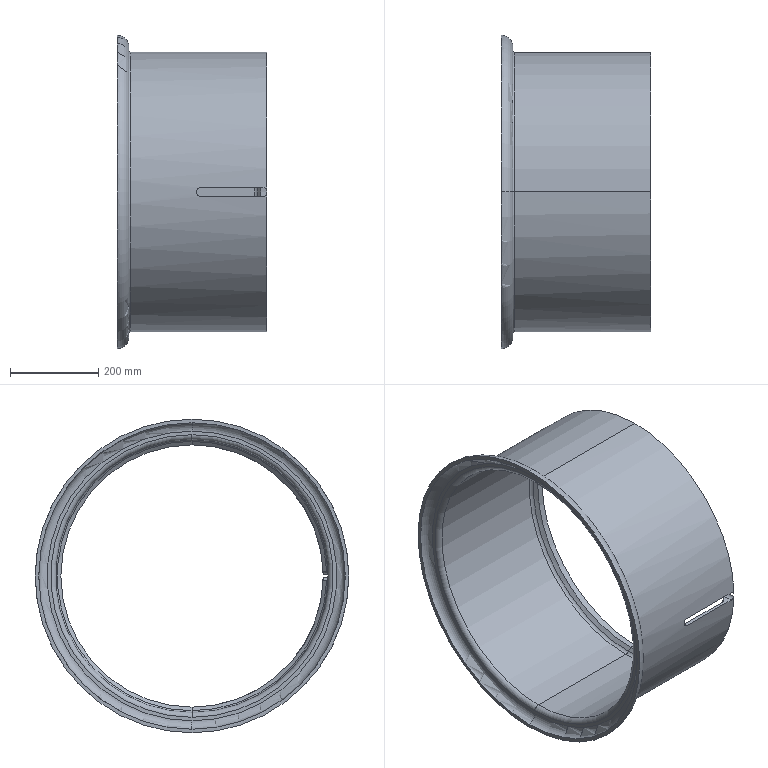Part | SolidWorks | features Fillet 2, ICE 1, Revolution 1 | 1 solid | 30 faces | box 340 x 711 x 711 mm | volume 6226699 mm3 | torus 11 | cylinder 10 | plane 6 | cone 3 | commonest cylinder face diameters 20 x3 595 x3 619 x2 635 x2
STEP:
#1=CARTESIAN_POINT('',(27.,0.,-320.5));
#2=VERTEX_POINT('',#1);
#3=CARTESIAN_POINT('',(27.,0.,320.5));
#4=VERTEX_POINT('',#3);
#5=CARTESIAN_POINT('',(27.,0.,0.));
#6=DIRECTION('',(-1.,0.,0.));
#7=DIRECTION('',(0.,0.,1.));
#8=AXIS2_PLACEMENT_3D('',#5,#6,#7);
#9=CIRCLE('',#8,320.5);
#10=EDGE_CURVE('',#2,#4,#9,.T.);
#11=ORIENTED_EDGE('',*,*,#10,.F.);
#12=CARTESIAN_POINT('',(30.,0.,-317.5));
#13=VERTEX_POINT('',#12);
#14=CARTESIAN_POINT('',(30.,0.,-320.5));
#15=DIRECTION('',(0.,1.,0.));
#16=DIRECTION('',(0.,0.,1.));
#17=AXIS2_PLACEMENT_3D('',#14,#15,#16);
#18=CIRCLE('',#17,3.);
#19=EDGE_CURVE('',#2,#13,#18,.T.);
#20=ORIENTED_EDGE('',*,*,#19,.T.);
#21=CARTESIAN_POINT('',(30.,0.,317.5));
#22=VERTEX_POINT('',#21);
#23=CARTESIAN_POINT('',(30.,0.,0.));
#24=DIRECTION('',(1.,0.,0.));
#25=DIRECTION('',(0.,0.,1.));
#26=AXIS2_PLACEMENT_3D('',#23,#24,#25);
#27=CIRCLE('',#26,317.5);
#28=EDGE_CURVE('',#22,#13,#27,.T.);
#29=ORIENTED_EDGE('',*,*,#28,.F.);
#30=CARTESIAN_POINT('',(30.,0.,320.5));
#31=DIRECTION('',(0.,-1.,0.));
#32=DIRECTION('',(0.,0.,-1.));
#33=AXIS2_PLACEMENT_3D('',#30,#31,#32);
#34=CIRCLE('',#33,3.);
#35=EDGE_CURVE('',#4,#22,#34,.T.);
#36=ORIENTED_EDGE('',*,*,#35,.F.);
#37=EDGE_LOOP('',(#11,#20,#29,#36));
#38=FACE_OUTER_BOUND('',#37,.T.);
#39=CARTESIAN_POINT('',(30.,0.,0.));
#40=DIRECTION('',(-1.,0.,0.));
#41=DIRECTION('',(0.,0.,1.));
#42=AXIS2_PLACEMENT_3D('',#39,#40,#41);
#43=TOROIDAL_SURFACE('',#42,320.5,3.);
#44=ADVANCED_FACE('',(#38),#43,.F.);
#45=CARTESIAN_POINT('',(319.298,0.,-305.542));
#46=VERTEX_POINT('',#45);
#47=CARTESIAN_POINT('',(319.298,-305.378,-10.));
#48=VERTEX_POINT('',#47);
#49=CARTESIAN_POINT('',(319.298,0.,0.));
#50=DIRECTION('',(-1.,0.,0.));
#51=DIRECTION('',(0.,0.,1.));
#52=AXIS2_PLACEMENT_3D('',#49,#50,#51);
#53=CIRCLE('',#52,305.542);
#54=EDGE_CURVE('',#46,#48,#53,.T.);
#55=ORIENTED_EDGE('',*,*,#54,.F.);
#56=CARTESIAN_POINT('',(310.848,0.,-309.5));
#57=VERTEX_POINT('',#56);
#58=CARTESIAN_POINT('',(310.848,0.,-298.5));
#59=DIRECTION('',(0.,1.,0.));
#60=DIRECTION('',(0.,0.,1.));
#61=AXIS2_PLACEMENT_3D('',#58,#59,#60);
#62=CIRCLE('',#61,11.);
#63=EDGE_CURVE('',#46,#57,#62,.T.);
#64=ORIENTED_EDGE('',*,*,#63,.T.);
#65=CARTESIAN_POINT('',(310.848,-309.338,-10.));
#66=VERTEX_POINT('',#65);
#67=CARTESIAN_POINT('',(310.848,0.,0.));
#68=DIRECTION('',(1.,0.,0.));
#69=DIRECTION('',(0.,0.,1.));
#70=AXIS2_PLACEMENT_3D('',#67,#68,#69);
#71=CIRCLE('',#70,309.5);
#72=EDGE_CURVE('',#66,#57,#71,.T.);
#73=ORIENTED_EDGE('',*,*,#72,.F.);
#74=CARTESIAN_POINT('',(310.848,-309.338,-10.));
#75=CARTESIAN_POINT('',(311.247,-309.338,-10.));
#76=CARTESIAN_POINT('',(311.646,-309.317,-10.));
#77=CARTESIAN_POINT('',(312.444,-309.229,-10.));
#78=CARTESIAN_POINT('',(312.845,-309.163,-10.));
#79=CARTESIAN_POINT('',(313.632,-308.988,-10.));
#80=CARTESIAN_POINT('',(314.02,-308.879,-10.));
#81=CARTESIAN_POINT('',(314.783,-308.618,-10.));
#82=CARTESIAN_POINT('',(315.16,-308.466,-10.));
#83=CARTESIAN_POINT('',(316.25,-307.954,-10.));
#84=CARTESIAN_POINT('',(316.931,-307.538,-10.));
#85=CARTESIAN_POINT('',(317.885,-306.802,-10.));
#86=CARTESIAN_POINT('',(318.192,-306.536,-10.));
#87=CARTESIAN_POINT('',(318.771,-305.978,-10.));
#88=CARTESIAN_POINT('',(319.043,-305.685,-10.));
#89=CARTESIAN_POINT('',(319.298,-305.378,-10.));
#90=B_SPLINE_CURVE_WITH_KNOTS('',3,(#74,#75,#76,#77,#78,#79,#80,#81,#82,#83,#84,#85,#86,#87,#88,#89),.UNSPECIFIED.,.F.,.F.,(4,2,2,2,2,2,2,4),(0.06468,0.06588,0.06708,0.06827,0.06947,0.07187,0.07306,0.07426),.UNSPECIFIED.);
#91=EDGE_CURVE('',#66,#48,#90,.T.);
#92=ORIENTED_EDGE('',*,*,#91,.T.);
#93=EDGE_LOOP('',(#55,#64,#73,#92));
#94=FACE_OUTER_BOUND('',#93,.T.);
#95=CARTESIAN_POINT('',(310.848,0.,0.));
#96=DIRECTION('',(-1.,0.,0.));
#97=DIRECTION('',(0.,0.,1.));
#98=AXIS2_PLACEMENT_3D('',#95,#96,#97);
#99=TOROIDAL_SURFACE('',#98,298.5,11.);
#100=ADVANCED_FACE('',(#94),#99,.F.);
#101=ORIENTED_EDGE('',*,*,#63,.F.);
#102=CARTESIAN_POINT('',(319.298,0.,305.542));
#103=VERTEX_POINT('',#102);
#104=CARTESIAN_POINT('',(319.298,0.,0.));
#105=DIRECTION('',(-1.,0.,0.));
#106=DIRECTION('',(0.,0.,1.));
#107=AXIS2_PLACEMENT_3D('',#104,#105,#106);
#108=CIRCLE('',#107,305.542);
#109=EDGE_CURVE('',#103,#46,#108,.T.);
#110=ORIENTED_EDGE('',*,*,#109,.F.);
#111=CARTESIAN_POINT('',(310.848,0.,309.5));
#112=VERTEX_POINT('',#111);
#113=CARTESIAN_POINT('',(310.848,0.,298.5));
#114=DIRECTION('',(0.,-1.,0.));
#115=DIRECTION('',(0.,0.,-1.));
#116=AXIS2_PLACEMENT_3D('',#113,#114,#115);
#117=CIRCLE('',#116,11.);
#118=EDGE_CURVE('',#103,#112,#117,.T.);
#119=ORIENTED_EDGE('',*,*,#118,.T.);
#120=CARTESIAN_POINT('',(310.848,0.,0.));
#121=DIRECTION('',(1.,0.,0.));
#122=DIRECTION('',(0.,0.,1.));
#123=AXIS2_PLACEMENT_3D('',#120,#121,#122);
#124=CIRCLE('',#123,309.5);
#125=EDGE_CURVE('',#57,#112,#124,.T.);
#126=ORIENTED_EDGE('',*,*,#125,.F.);
#127=EDGE_LOOP('',(#101,#110,#119,#126));
#128=FACE_OUTER_BOUND('',#127,.T.);
#129=CARTESIAN_POINT('',(310.848,0.,0.));
#130=DIRECTION('',(-1.,0.,0.));
#131=DIRECTION('',(0.,0.,1.));
#132=AXIS2_PLACEMENT_3D('',#129,#130,#131);
#133=TOROIDAL_SURFACE('',#132,298.5,11.);
#134=ADVANCED_FACE('',(#128),#133,.F.);
#135=CARTESIAN_POINT('',(30.,0.,309.5));
#136=VERTEX_POINT('',#135);
#137=CARTESIAN_POINT('',(30.,0.,-309.5));
#138=VERTEX_POINT('',#137);
#139=CARTESIAN_POINT('',(30.,0.,0.));
#140=DIRECTION('',(-1.,0.,0.));
#141=DIRECTION('',(0.,0.,-1.));
#142=AXIS2_PLACEMENT_3D('',#139,#140,#141);
#143=CIRCLE('',#142,309.5);
#144=EDGE_CURVE('',#136,#138,#143,.T.);
#145=ORIENTED_EDGE('',*,*,#144,.F.);
#146=CARTESIAN_POINT('',(19.,0.,320.5));
#147=VERTEX_POINT('',#146);
#148=CARTESIAN_POINT('',(30.,0.,320.5));
#149=DIRECTION('',(0.,1.,0.));
#150=DIRECTION('',(0.,0.,1.));
#151=AXIS2_PLACEMENT_3D('',#148,#149,#150);
#152=CIRCLE('',#151,11.);
#153=EDGE_CURVE('',#136,#147,#152,.T.);
#154=ORIENTED_EDGE('',*,*,#153,.T.);
#155=CARTESIAN_POINT('',(19.,0.,-320.5));
#156=VERTEX_POINT('',#155);
#157=CARTESIAN_POINT('',(19.,0.,0.));
#158=DIRECTION('',(1.,0.,0.));
#159=DIRECTION('',(0.,0.,-1.));
#160=AXIS2_PLACEMENT_3D('',#157,#158,#159);
#161=CIRCLE('',#160,320.5);
#162=EDGE_CURVE('',#156,#147,#161,.T.);
#163=ORIENTED_EDGE('',*,*,#162,.F.);
#164=CARTESIAN_POINT('',(30.,0.,-320.5));
#165=DIRECTION('',(0.,-1.,0.));
#166=DIRECTION('',(0.,0.,-1.));
#167=AXIS2_PLACEMENT_3D('',#164,#165,#166);
#168=CIRCLE('',#167,11.);
#169=EDGE_CURVE('',#138,#156,#168,.T.);
#170=ORIENTED_EDGE('',*,*,#169,.F.);
#171=EDGE_LOOP('',(#145,#154,#163,#170));
#172=FACE_OUTER_BOUND('',#171,.T.);
#173=CARTESIAN_POINT('',(30.,0.,0.));
#174=DIRECTION('',(1.,0.,0.));
#175=DIRECTION('',(0.,0.,-1.));
#176=AXIS2_PLACEMENT_3D('',#173,#174,#175);
#177=TOROIDAL_SURFACE('',#176,320.5,11.);
#178=ADVANCED_FACE('',(#172),#177,.T.);
#179=CARTESIAN_POINT('',(340.,0.,317.5));
#180=VERTEX_POINT('',#179);
#181=CARTESIAN_POINT('',(340.,0.,-317.5));
#182=VERTEX_POINT('',#181);
#183=CARTESIAN_POINT('',(340.,0.,0.));
#184=DIRECTION('',(-1.,0.,0.));
#185=DIRECTION('',(0.,0.,1.));
#186=AXIS2_PLACEMENT_3D('',#183,#184,#185);
#187=CIRCLE('',#186,317.5);
#188=EDGE_CURVE('',#180,#182,#187,.T.);
#189=ORIENTED_EDGE('',*,*,#188,.T.);
#190=CARTESIAN_POINT('',(-326.853,0.,-317.5));
#191=DIRECTION('',(-1.,0.,0.));
#192=VECTOR('',#191,1000.);
#193=LINE('',#190,#192);
#194=EDGE_CURVE('',#182,#13,#193,.T.);
#195=ORIENTED_EDGE('',*,*,#194,.T.);
#196=CARTESIAN_POINT('',(30.,0.,0.));
#197=DIRECTION('',(1.,0.,0.));
#198=DIRECTION('',(0.,0.,1.));
#199=AXIS2_PLACEMENT_3D('',#196,#197,#198);
#200=CIRCLE('',#199,317.5);
#201=EDGE_CURVE('',#13,#22,#200,.T.);
#202=ORIENTED_EDGE('',*,*,#201,.T.);
#203=CARTESIAN_POINT('',(-326.853,0.,317.5));
#204=DIRECTION('',(-1.,0.,0.));
#205=VECTOR('',#204,1000.);
#206=LINE('',#203,#205);
#207=EDGE_CURVE('',#180,#22,#206,.T.);
#208=ORIENTED_EDGE('',*,*,#207,.F.);
#209=EDGE_LOOP('',(#189,#195,#202,#208));
#210=FACE_OUTER_BOUND('',#209,.T.);
#211=CARTESIAN_POINT('',(-326.853,0.,0.));
#212=DIRECTION('',(-1.,0.,0.));
#213=DIRECTION('',(0.,0.,1.));
#214=AXIS2_PLACEMENT_3D('',#211,#212,#213);
#215=CYLINDRICAL_SURFACE('',#214,317.5);
#216=ADVANCED_FACE('',(#210),#215,.T.);
#217=CARTESIAN_POINT('',(340.,0.,-297.5));
#218=VERTEX_POINT('',#217);
#219=CARTESIAN_POINT('',(340.,-297.468,-4.359));
#220=VERTEX_POINT('',#219);
#221=CARTESIAN_POINT('',(340.,0.,0.));
#222=DIRECTION('',(-1.,0.,0.));
#223=DIRECTION('',(0.,0.,1.));
#224=AXIS2_PLACEMENT_3D('',#221,#222,#223);
#225=CIRCLE('',#224,297.5);
#226=EDGE_CURVE('',#218,#220,#225,.T.);
#227=ORIENTED_EDGE('',*,*,#226,.F.);
#228=CARTESIAN_POINT('',(326.,0.,-297.5));
#229=VERTEX_POINT('',#228);
#230=CARTESIAN_POINT('',(-326.853,0.,-297.5));
#231=DIRECTION('',(-1.,0.,0.));
#232=VECTOR('',#231,1000.);
#233=LINE('',#230,#232);
#234=EDGE_CURVE('',#218,#229,#233,.T.);
#235=ORIENTED_EDGE('',*,*,#234,.T.);
#236=CARTESIAN_POINT('',(326.,-297.332,-10.));
#237=VERTEX_POINT('',#236);
#238=CARTESIAN_POINT('',(326.,0.,0.));
#239=DIRECTION('',(-1.,0.,0.));
#240=DIRECTION('',(0.,0.,1.));
#241=AXIS2_PLACEMENT_3D('',#238,#239,#240);
#242=CIRCLE('',#241,297.5);
#243=EDGE_CURVE('',#229,#237,#242,.T.);
#244=ORIENTED_EDGE('',*,*,#243,.T.);
#245=CARTESIAN_POINT('',(331.,-297.332,-10.));
#246=VERTEX_POINT('',#245);
#247=CARTESIAN_POINT('',(-326.853,-297.332,-10.));
#248=DIRECTION('',(1.,0.,0.));
#249=VECTOR('',#248,1000.);
#250=LINE('',#247,#249);
#251=EDGE_CURVE('',#237,#246,#250,.T.);
#252=ORIENTED_EDGE('',*,*,#251,.T.);
#253=CARTESIAN_POINT('',(331.,-297.332,-10.));
#254=CARTESIAN_POINT('',(331.941,-297.332,-10.));
#255=CARTESIAN_POINT('',(332.861,-297.336,-9.87));
#256=CARTESIAN_POINT('',(334.207,-297.349,-9.483));
#257=CARTESIAN_POINT('',(334.651,-297.354,-9.321));
#258=CARTESIAN_POINT('',(335.502,-297.366,-8.941));
#259=CARTESIAN_POINT('',(335.911,-297.372,-8.723));
#260=CARTESIAN_POINT('',(336.699,-297.386,-8.23));
#261=CARTESIAN_POINT('',(337.08,-297.394,-7.954));
#262=CARTESIAN_POINT('',(337.797,-297.409,-7.35));
#263=CARTESIAN_POINT('',(338.131,-297.417,-7.026));
#264=CARTESIAN_POINT('',(338.751,-297.433,-6.336));
#265=CARTESIAN_POINT('',(339.037,-297.44,-5.969));
#266=CARTESIAN_POINT('',(339.559,-297.455,-5.192));
#267=CARTESIAN_POINT('',(339.795,-297.462,-4.782));
#268=CARTESIAN_POINT('',(340.,-297.468,-4.359));
#269=B_SPLINE_CURVE_WITH_KNOTS('',3,(#253,#254,#255,#256,#257,#258,#259,#260,#261,#262,#263,#264,#265,#266,#267,#268),.UNSPECIFIED.,.F.,.F.,(4,2,2,2,2,2,2,4),(0.,0.002784,0.004176,0.005568,0.00696,0.008352,0.009744,0.01114),.UNSPECIFIED.);
#270=EDGE_CURVE('',#246,#220,#269,.T.);
#271=ORIENTED_EDGE('',*,*,#270,.T.);
#272=EDGE_LOOP('',(#227,#235,#244,#252,#271));
#273=FACE_OUTER_BOUND('',#272,.T.);
#274=CARTESIAN_POINT('',(-326.853,0.,0.));
#275=DIRECTION('',(-1.,0.,0.));
#276=DIRECTION('',(0.,0.,1.));
#277=AXIS2_PLACEMENT_3D('',#274,#275,#276);
#278=CYLINDRICAL_SURFACE('',#277,297.5);
#279=ADVANCED_FACE('',(#273),#278,.F.);
#280=ORIENTED_EDGE('',*,*,#234,.F.);
#281=CARTESIAN_POINT('',(340.,0.,297.5));
#282=VERTEX_POINT('',#281);
#283=CARTESIAN_POINT('',(340.,0.,0.));
#284=DIRECTION('',(-1.,0.,0.));
#285=DIRECTION('',(0.,0.,1.));
#286=AXIS2_PLACEMENT_3D('',#283,#284,#285);
#287=CIRCLE('',#286,297.5);
#288=EDGE_CURVE('',#282,#218,#287,.T.);
#289=ORIENTED_EDGE('',*,*,#288,.F.);
#290=CARTESIAN_POINT('',(326.,0.,297.5));
#291=VERTEX_POINT('',#290);
#292=CARTESIAN_POINT('',(-326.853,0.,297.5));
#293=DIRECTION('',(-1.,0.,0.));
#294=VECTOR('',#293,1000.);
#295=LINE('',#292,#294);
#296=EDGE_CURVE('',#282,#291,#295,.T.);
#297=ORIENTED_EDGE('',*,*,#296,.T.);
#298=CARTESIAN_POINT('',(326.,0.,0.));
#299=DIRECTION('',(-1.,0.,0.));
#300=DIRECTION('',(0.,0.,1.));
#301=AXIS2_PLACEMENT_3D('',#298,#299,#300);
#302=CIRCLE('',#301,297.5);
#303=EDGE_CURVE('',#291,#229,#302,.T.);
#304=ORIENTED_EDGE('',*,*,#303,.T.);
#305=EDGE_LOOP('',(#280,#289,#297,#304));
#306=FACE_OUTER_BOUND('',#305,.T.);
#307=CARTESIAN_POINT('',(-326.853,0.,0.));
#308=DIRECTION('',(-1.,0.,0.));
#309=DIRECTION('',(0.,0.,1.));
#310=AXIS2_PLACEMENT_3D('',#307,#308,#309);
#311=CYLINDRICAL_SURFACE('',#310,297.5);
#312=ADVANCED_FACE('',(#306),#311,.F.);
#313=ORIENTED_EDGE('',*,*,#243,.F.);
#314=CARTESIAN_POINT('',(316.,0.,-309.5));
#315=DIRECTION('',(-0.6402,0.,-0.7682));
#316=VECTOR('',#315,1000.);
#317=LINE('',#314,#316);
#318=EDGE_CURVE('',#229,#46,#317,.T.);
#319=ORIENTED_EDGE('',*,*,#318,.T.);
#320=ORIENTED_EDGE('',*,*,#54,.T.);
#321=CARTESIAN_POINT('',(319.298,-305.378,-10.));
#322=CARTESIAN_POINT('',(321.532,-302.696,-10.));
#323=CARTESIAN_POINT('',(323.766,-300.014,-10.));
#324=CARTESIAN_POINT('',(326.,-297.332,-10.));
#325=B_SPLINE_CURVE_WITH_KNOTS('',3,(#321,#322,#323,#324),.UNSPECIFIED.,.F.,.F.,(4,4),(0.287,0.2975),.UNSPECIFIED.);
#326=EDGE_CURVE('',#48,#237,#325,.T.);
#327=ORIENTED_EDGE('',*,*,#326,.T.);
#328=EDGE_LOOP('',(#313,#319,#320,#327));
#329=FACE_OUTER_BOUND('',#328,.T.);
#330=CARTESIAN_POINT('',(316.,0.,0.));
#331=DIRECTION('',(-1.,0.,0.));
#332=DIRECTION('',(0.,0.,1.));
#333=AXIS2_PLACEMENT_3D('',#330,#331,#332);
#334=CONICAL_SURFACE('',#333,309.5,0.8761);
#335=ADVANCED_FACE('',(#329),#334,.F.);
#336=ORIENTED_EDGE('',*,*,#318,.F.);
#337=ORIENTED_EDGE('',*,*,#303,.F.);
#338=CARTESIAN_POINT('',(316.,0.,309.5));
#339=DIRECTION('',(-0.6402,0.,0.7682));
#340=VECTOR('',#339,1000.);
#341=LINE('',#338,#340);
#342=EDGE_CURVE('',#291,#103,#341,.T.);
#343=ORIENTED_EDGE('',*,*,#342,.T.);
#344=ORIENTED_EDGE('',*,*,#109,.T.);
#345=EDGE_LOOP('',(#336,#337,#343,#344));
#346=FACE_OUTER_BOUND('',#345,.T.);
#347=CARTESIAN_POINT('',(316.,0.,0.));
#348=DIRECTION('',(-1.,0.,0.));
#349=DIRECTION('',(0.,0.,1.));
#350=AXIS2_PLACEMENT_3D('',#347,#348,#349);
#351=CONICAL_SURFACE('',#350,309.5,0.8761);
#352=ADVANCED_FACE('',(#346),#351,.F.);
#353=ORIENTED_EDGE('',*,*,#72,.T.);
#354=CARTESIAN_POINT('',(-326.853,0.,-309.5));
#355=DIRECTION('',(-1.,0.,0.));
#356=VECTOR('',#355,1000.);
#357=LINE('',#354,#356);
#358=EDGE_CURVE('',#57,#138,#357,.T.);
#359=ORIENTED_EDGE('',*,*,#358,.T.);
#360=CARTESIAN_POINT('',(30.,0.,0.));
#361=DIRECTION('',(-1.,0.,0.));
#362=DIRECTION('',(0.,0.,-1.));
#363=AXIS2_PLACEMENT_3D('',#360,#361,#362);
#364=CIRCLE('',#363,309.5);
#365=EDGE_CURVE('',#138,#136,#364,.T.);
#366=ORIENTED_EDGE('',*,*,#365,.T.);
#367=CARTESIAN_POINT('',(-326.853,0.,309.5));
#368=DIRECTION('',(-1.,0.,0.));
#369=VECTOR('',#368,1000.);
#370=LINE('',#367,#369);
#371=EDGE_CURVE('',#112,#136,#370,.T.);
#372=ORIENTED_EDGE('',*,*,#371,.F.);
#373=CARTESIAN_POINT('',(310.848,-309.338,10.));
#374=VERTEX_POINT('',#373);
#375=CARTESIAN_POINT('',(310.848,0.,0.));
#376=DIRECTION('',(1.,0.,0.));
#377=DIRECTION('',(0.,0.,1.));
#378=AXIS2_PLACEMENT_3D('',#375,#376,#377);
#379=CIRCLE('',#378,309.5);
#380=EDGE_CURVE('',#112,#374,#379,.T.);
#381=ORIENTED_EDGE('',*,*,#380,.T.);
#382=CARTESIAN_POINT('',(190.,-309.338,10.));
#383=VERTEX_POINT('',#382);
#384=CARTESIAN_POINT('',(-326.853,-309.338,10.));
#385=DIRECTION('',(-1.,0.,0.));
#386=VECTOR('',#385,1000.);
#387=LINE('',#384,#386);
#388=EDGE_CURVE('',#374,#383,#387,.T.);
#389=ORIENTED_EDGE('',*,*,#388,.T.);
#390=CARTESIAN_POINT('',(190.,-309.338,-10.));
#391=VERTEX_POINT('',#390);
#392=CARTESIAN_POINT('',(190.,-309.338,10.));
#393=CARTESIAN_POINT('',(189.339,-309.338,10.));
#394=CARTESIAN_POINT('',(188.69,-309.341,9.935));
#395=CARTESIAN_POINT('',(187.731,-309.347,9.745));
#396=CARTESIAN_POINT('',(187.414,-309.349,9.666));
#397=CARTESIAN_POINT('',(186.786,-309.355,9.475));
#398=CARTESIAN_POINT('',(186.474,-309.358,9.363));
#399=CARTESIAN_POINT('',(185.566,-309.37,8.987));
#400=CARTESIAN_POINT('',(184.992,-309.378,8.68));
#401=CARTESIAN_POINT('',(184.176,-309.393,8.136));
#402=CARTESIAN_POINT('',(183.912,-309.398,7.94));
#403=CARTESIAN_POINT('',(183.402,-309.409,7.522));
#404=CARTESIAN_POINT('',(183.159,-309.414,7.302));
#405=CARTESIAN_POINT('',(182.468,-309.43,6.61));
#406=CARTESIAN_POINT('',(182.054,-309.44,6.106));
#407=CARTESIAN_POINT('',(181.505,-309.455,5.287));
#408=CARTESIAN_POINT('',(181.335,-309.46,5.003));
#409=CARTESIAN_POINT('',(181.027,-309.468,4.426));
#410=CARTESIAN_POINT('',(180.748,-309.477,3.836));
#411=CARTESIAN_POINT('',(180.528,-309.483,3.222));
#412=CARTESIAN_POINT('',(180.337,-309.489,2.597));
#413=CARTESIAN_POINT('',(180.257,-309.492,2.276));
#414=CARTESIAN_POINT('',(180.064,-309.498,1.308));
#415=CARTESIAN_POINT('',(180.,-309.5,0.6589));
#416=CARTESIAN_POINT('',(180.,-309.5,-0.3193));
#417=CARTESIAN_POINT('',(180.015,-309.499,-0.6462));
#418=CARTESIAN_POINT('',(180.08,-309.497,-1.302));
#419=CARTESIAN_POINT('',(180.128,-309.496,-1.628));
#420=CARTESIAN_POINT('',(180.319,-309.49,-2.59));
#421=CARTESIAN_POINT('',(180.508,-309.484,-3.214));
#422=CARTESIAN_POINT('',(180.883,-309.473,-4.122));
#423=CARTESIAN_POINT('',(181.024,-309.469,-4.421));
#424=CARTESIAN_POINT('',(181.334,-309.46,-5.001));
#425=CARTESIAN_POINT('',(181.502,-309.455,-5.281));
#426=CARTESIAN_POINT('',(182.044,-309.44,-6.094));
#427=CARTESIAN_POINT('',(182.457,-309.43,-6.599));
#428=CARTESIAN_POINT('',(183.39,-309.409,-7.533));
#429=CARTESIAN_POINT('',(183.896,-309.398,-7.948));
#430=CARTESIAN_POINT('',(184.708,-309.384,-8.491));
#431=CARTESIAN_POINT('',(184.988,-309.379,-8.659));
#432=CARTESIAN_POINT('',(185.566,-309.37,-8.969));
#433=CARTESIAN_POINT('',(185.865,-309.366,-9.111));
#434=CARTESIAN_POINT('',(186.774,-309.355,-9.488));
#435=CARTESIAN_POINT('',(187.397,-309.349,-9.677));
#436=CARTESIAN_POINT('',(188.678,-309.341,-9.934));
#437=CARTESIAN_POINT('',(189.339,-309.338,-10.));
#438=CARTESIAN_POINT('',(190.,-309.338,-10.));
#439=B_SPLINE_CURVE_WITH_KNOTS('',3,(#392,#393,#394,#395,#396,#397,#398,#399,#400,#401,#402,#403,#404,#405,#406,#407,#408,#409,#410,#411,#412,#413,#414,#415,#416,#417,#418,#419,#420,#421,#422,#423,#424,#425,#426,#427,#428,#429,#430,#431,#432,#433,#434,#435,#436,#437,#438),.UNSPECIFIED.,.F.,.F.,(4,2,2,2,2,2,2,2,2,1,2,2,2,2,2,2,2,2,2,2,2,2,2,4),(0.,0.001954,0.002931,0.003908,0.005861,0.006838,0.007815,0.009769,0.01075,0.01172,0.0127,0.01368,0.01563,0.01661,0.01758,0.01954,0.02051,0.02149,0.02345,0.0254,0.02638,0.02735,0.02931,0.03126),.UNSPECIFIED.);
#440=EDGE_CURVE('',#383,#391,#439,.T.);
#441=ORIENTED_EDGE('',*,*,#440,.T.);
#442=CARTESIAN_POINT('',(-326.853,-309.338,-10.));
#443=DIRECTION('',(1.,0.,0.));
#444=VECTOR('',#443,1000.);
#445=LINE('',#442,#444);
#446=EDGE_CURVE('',#391,#66,#445,.T.);
#447=ORIENTED_EDGE('',*,*,#446,.T.);
#448=EDGE_LOOP('',(#353,#359,#366,#372,#381,#389,#441,#447));
#449=FACE_OUTER_BOUND('',#448,.T.);
#450=CARTESIAN_POINT('',(-326.853,0.,0.));
#451=DIRECTION('',(-1.,0.,0.));
#452=DIRECTION('',(0.,0.,1.));
#453=AXIS2_PLACEMENT_3D('',#450,#451,#452);
#454=CYLINDRICAL_SURFACE('',#453,309.5);
#455=ADVANCED_FACE('',(#449),#454,.F.);
#456=CARTESIAN_POINT('',(19.,0.,-328.5));
#457=VERTEX_POINT('',#456);
#458=CARTESIAN_POINT('',(19.,0.,328.5));
#459=VERTEX_POINT('',#458);
#460=CARTESIAN_POINT('',(19.,0.,0.));
#461=DIRECTION('',(-1.,0.,0.));
#462=DIRECTION('',(0.,0.,1.));
#463=AXIS2_PLACEMENT_3D('',#460,#461,#462);
#464=CIRCLE('',#463,328.5);
#465=EDGE_CURVE('',#457,#459,#464,.T.);
#466=ORIENTED_EDGE('',*,*,#465,.F.);
#467=CARTESIAN_POINT('',(0.,0.,-347.5));
#468=VERTEX_POINT('',#467);
#469=CARTESIAN_POINT('',(0.,0.,-328.5));
#470=DIRECTION('',(0.,1.,0.));
#471=DIRECTION('',(0.,0.,1.));
#472=AXIS2_PLACEMENT_3D('',#469,#470,#471);
#473=CIRCLE('',#472,19.);
#474=EDGE_CURVE('',#457,#468,#473,.T.);
#475=ORIENTED_EDGE('',*,*,#474,.T.);
#476=CARTESIAN_POINT('',(0.,0.,347.5));
#477=VERTEX_POINT('',#476);
#478=CARTESIAN_POINT('',(0.,0.,0.));
#479=DIRECTION('',(-1.,0.,0.));
#480=DIRECTION('',(0.,0.,1.));
#481=AXIS2_PLACEMENT_3D('',#478,#479,#480);
#482=CIRCLE('',#481,347.5);
#483=EDGE_CURVE('',#468,#477,#482,.T.);
#484=ORIENTED_EDGE('',*,*,#483,.T.);
#485=CARTESIAN_POINT('',(0.,0.,328.5));
#486=DIRECTION('',(0.,-1.,0.));
#487=DIRECTION('',(0.,0.,-1.));
#488=AXIS2_PLACEMENT_3D('',#485,#486,#487);
#489=CIRCLE('',#488,19.);
#490=EDGE_CURVE('',#459,#477,#489,.T.);
#491=ORIENTED_EDGE('',*,*,#490,.F.);
#492=EDGE_LOOP('',(#466,#475,#484,#491));
#493=FACE_OUTER_BOUND('',#492,.T.);
#494=CARTESIAN_POINT('',(0.,0.,0.));
#495=DIRECTION('',(-1.,0.,0.));
#496=DIRECTION('',(0.,0.,1.));
#497=AXIS2_PLACEMENT_3D('',#494,#495,#496);
#498=TOROIDAL_SURFACE('',#497,328.5,19.);
#499=ADVANCED_FACE('',(#493),#498,.F.);
#500=CARTESIAN_POINT('',(27.,0.,328.5));
#501=VERTEX_POINT('',#500);
#502=CARTESIAN_POINT('',(27.,0.,-328.5));
#503=VERTEX_POINT('',#502);
#504=CARTESIAN_POINT('',(27.,0.,0.));
#505=DIRECTION('',(-1.,0.,0.));
#506=DIRECTION('',(0.,0.,1.));
#507=AXIS2_PLACEMENT_3D('',#504,#505,#506);
#508=CIRCLE('',#507,328.5);
#509=EDGE_CURVE('',#501,#503,#508,.T.);
#510=ORIENTED_EDGE('',*,*,#509,.T.);
#511=CARTESIAN_POINT('',(0.,0.,-355.5));
#512=VERTEX_POINT('',#511);
#513=CARTESIAN_POINT('',(0.,0.,-328.5));
#514=DIRECTION('',(0.,1.,0.));
#515=DIRECTION('',(0.,0.,1.));
#516=AXIS2_PLACEMENT_3D('',#513,#514,#515);
#517=CIRCLE('',#516,27.);
#518=EDGE_CURVE('',#503,#512,#517,.T.);
#519=ORIENTED_EDGE('',*,*,#518,.T.);
#520=CARTESIAN_POINT('',(0.,0.,355.5));
#521=VERTEX_POINT('',#520);
#522=CARTESIAN_POINT('',(0.,0.,0.));
#523=DIRECTION('',(-1.,0.,0.));
#524=DIRECTION('',(0.,0.,1.));
#525=AXIS2_PLACEMENT_3D('',#522,#523,#524);
#526=CIRCLE('',#525,355.5);
#527=EDGE_CURVE('',#521,#512,#526,.T.);
#528=ORIENTED_EDGE('',*,*,#527,.F.);
#529=CARTESIAN_POINT('',(0.,0.,328.5));
#530=DIRECTION('',(0.,-1.,0.));
#531=DIRECTION('',(0.,0.,-1.));
#532=AXIS2_PLACEMENT_3D('',#529,#530,#531);
#533=CIRCLE('',#532,27.);
#534=EDGE_CURVE('',#501,#521,#533,.T.);
#535=ORIENTED_EDGE('',*,*,#534,.F.);
#536=EDGE_LOOP('',(#510,#519,#528,#535));
#537=FACE_OUTER_BOUND('',#536,.T.);
#538=CARTESIAN_POINT('',(0.,0.,0.));
#539=DIRECTION('',(-1.,0.,0.));
#540=DIRECTION('',(0.,0.,1.));
#541=AXIS2_PLACEMENT_3D('',#538,#539,#540);
#542=TOROIDAL_SURFACE('',#541,328.5,27.);
#543=ADVANCED_FACE('',(#537),#542,.T.);
#544=ORIENTED_EDGE('',*,*,#518,.F.);
#545=CARTESIAN_POINT('',(27.,0.,0.));
#546=DIRECTION('',(-1.,0.,0.));
#547=DIRECTION('',(0.,0.,1.));
#548=AXIS2_PLACEMENT_3D('',#545,#546,#547);
#549=CIRCLE('',#548,328.5);
#550=EDGE_CURVE('',#503,#501,#549,.T.);
#551=ORIENTED_EDGE('',*,*,#550,.T.);
#552=ORIENTED_EDGE('',*,*,#534,.T.);
#553=CARTESIAN_POINT('',(0.,0.,0.));
#554=DIRECTION('',(-1.,0.,0.));
#555=DIRECTION('',(0.,0.,1.));
#556=AXIS2_PLACEMENT_3D('',#553,#554,#555);
#557=CIRCLE('',#556,355.5);
#558=EDGE_CURVE('',#512,#521,#557,.T.);
#559=ORIENTED_EDGE('',*,*,#558,.F.);
#560=EDGE_LOOP('',(#544,#551,#552,#559));
#561=FACE_OUTER_BOUND('',#560,.T.);
#562=CARTESIAN_POINT('',(0.,0.,0.));
#563=DIRECTION('',(-1.,0.,0.));
#564=DIRECTION('',(0.,0.,1.));
#565=AXIS2_PLACEMENT_3D('',#562,#563,#564);
#566=TOROIDAL_SURFACE('',#565,328.5,27.);
#567=ADVANCED_FACE('',(#561),#566,.T.);
#568=CARTESIAN_POINT('',(0.,0.,0.));
#569=DIRECTION('',(-1.,0.,0.));
#570=DIRECTION('',(0.,0.,1.));
#571=AXIS2_PLACEMENT_3D('',#568,#569,#570);
#572=CIRCLE('',#571,347.5);
#573=EDGE_CURVE('',#477,#468,#572,.T.);
#574=ORIENTED_EDGE('',*,*,#573,.F.);
#575=ORIENTED_EDGE('',*,*,#483,.F.);
#576=EDGE_LOOP('',(#574,#575));
#577=FACE_BOUND('',#576,.T.);
#578=ORIENTED_EDGE('',*,*,#527,.T.);
#579=ORIENTED_EDGE('',*,*,#558,.T.);
#580=EDGE_LOOP('',(#578,#579));
#581=FACE_OUTER_BOUND('',#580,.T.);
#582=CARTESIAN_POINT('',(0.,355.5,0.));
#583=DIRECTION('',(1.,0.,0.));
#584=DIRECTION('',(0.,0.,-1.));
#585=AXIS2_PLACEMENT_3D('',#582,#583,#584);
#586=PLANE('',#585);
#587=ADVANCED_FACE('',(#577,#581),#586,.F.);
#588=ORIENTED_EDGE('',*,*,#474,.F.);
#589=CARTESIAN_POINT('',(19.,0.,0.));
#590=DIRECTION('',(-1.,0.,0.));
#591=DIRECTION('',(0.,0.,1.));
#592=AXIS2_PLACEMENT_3D('',#589,#590,#591);
#593=CIRCLE('',#592,328.5);
#594=EDGE_CURVE('',#459,#457,#593,.T.);
#595=ORIENTED_EDGE('',*,*,#594,.F.);
#596=ORIENTED_EDGE('',*,*,#490,.T.);
#597=ORIENTED_EDGE('',*,*,#573,.T.);
#598=EDGE_LOOP('',(#588,#595,#596,#597));
#599=FACE_OUTER_BOUND('',#598,.T.);
#600=CARTESIAN_POINT('',(0.,0.,0.));
#601=DIRECTION('',(-1.,0.,0.));
#602=DIRECTION('',(0.,0.,1.));
#603=AXIS2_PLACEMENT_3D('',#600,#601,#602);
#604=TOROIDAL_SURFACE('',#603,328.5,19.);
#605=ADVANCED_FACE('',(#599),#604,.F.);
#606=ORIENTED_EDGE('',*,*,#162,.T.);
#607=CARTESIAN_POINT('',(19.,0.,0.));
#608=DIRECTION('',(1.,0.,0.));
#609=DIRECTION('',(0.,0.,-1.));
#610=AXIS2_PLACEMENT_3D('',#607,#608,#609);
#611=CIRCLE('',#610,320.5);
#612=EDGE_CURVE('',#147,#156,#611,.T.);
#613=ORIENTED_EDGE('',*,*,#612,.T.);
#614=EDGE_LOOP('',(#606,#613));
#615=FACE_BOUND('',#614,.T.);
#616=ORIENTED_EDGE('',*,*,#594,.T.);
#617=ORIENTED_EDGE('',*,*,#465,.T.);
#618=EDGE_LOOP('',(#616,#617));
#619=FACE_OUTER_BOUND('',#618,.T.);
#620=CARTESIAN_POINT('',(19.,328.5,0.));
#621=DIRECTION('',(1.,0.,0.));
#622=DIRECTION('',(0.,0.,-1.));
#623=AXIS2_PLACEMENT_3D('',#620,#621,#622);
#624=PLANE('',#623);
#625=ADVANCED_FACE('',(#615,#619),#624,.F.);
#626=ORIENTED_EDGE('',*,*,#358,.F.);
#627=ORIENTED_EDGE('',*,*,#125,.T.);
#628=ORIENTED_EDGE('',*,*,#371,.T.);
#629=ORIENTED_EDGE('',*,*,#144,.T.);
#630=EDGE_LOOP('',(#626,#627,#628,#629));
#631=FACE_OUTER_BOUND('',#630,.T.);
#632=CARTESIAN_POINT('',(-326.853,0.,0.));
#633=DIRECTION('',(-1.,0.,0.));
#634=DIRECTION('',(0.,0.,1.));
#635=AXIS2_PLACEMENT_3D('',#632,#633,#634);
#636=CYLINDRICAL_SURFACE('',#635,309.5);
#637=ADVANCED_FACE('',(#631),#636,.F.);
#638=ORIENTED_EDGE('',*,*,#342,.F.);
#639=CARTESIAN_POINT('',(326.,-297.332,10.));
#640=VERTEX_POINT('',#639);
#641=CARTESIAN_POINT('',(326.,0.,0.));
#642=DIRECTION('',(-1.,0.,0.));
#643=DIRECTION('',(0.,0.,1.));
#644=AXIS2_PLACEMENT_3D('',#641,#642,#643);
#645=CIRCLE('',#644,297.5);
#646=EDGE_CURVE('',#640,#291,#645,.T.);
#647=ORIENTED_EDGE('',*,*,#646,.F.);
#648=CARTESIAN_POINT('',(319.298,-305.378,10.));
#649=VERTEX_POINT('',#648);
#650=CARTESIAN_POINT('',(326.,-297.332,10.));
#651=CARTESIAN_POINT('',(323.766,-300.014,10.));
#652=CARTESIAN_POINT('',(321.532,-302.696,10.));
#653=CARTESIAN_POINT('',(319.298,-305.378,10.));
#654=B_SPLINE_CURVE_WITH_KNOTS('',3,(#650,#651,#652,#653),.UNSPECIFIED.,.F.,.F.,(4,4),(0.3392,0.3497),.UNSPECIFIED.);
#655=EDGE_CURVE('',#640,#649,#654,.T.);
#656=ORIENTED_EDGE('',*,*,#655,.T.);
#657=CARTESIAN_POINT('',(319.298,0.,0.));
#658=DIRECTION('',(-1.,0.,0.));
#659=DIRECTION('',(0.,0.,1.));
#660=AXIS2_PLACEMENT_3D('',#657,#658,#659);
#661=CIRCLE('',#660,305.542);
#662=EDGE_CURVE('',#649,#103,#661,.T.);
#663=ORIENTED_EDGE('',*,*,#662,.T.);
#664=EDGE_LOOP('',(#638,#647,#656,#663));
#665=FACE_OUTER_BOUND('',#664,.T.);
#666=CARTESIAN_POINT('',(316.,0.,0.));
#667=DIRECTION('',(-1.,0.,0.));
#668=DIRECTION('',(0.,0.,1.));
#669=AXIS2_PLACEMENT_3D('',#666,#667,#668);
#670=CONICAL_SURFACE('',#669,309.5,0.8761);
#671=ADVANCED_FACE('',(#665),#670,.F.);
#672=ORIENTED_EDGE('',*,*,#296,.F.);
#673=CARTESIAN_POINT('',(340.,-297.468,4.359));
#674=VERTEX_POINT('',#673);
#675=CARTESIAN_POINT('',(340.,0.,0.));
#676=DIRECTION('',(-1.,0.,0.));
#677=DIRECTION('',(0.,0.,1.));
#678=AXIS2_PLACEMENT_3D('',#675,#676,#677);
#679=CIRCLE('',#678,297.5);
#680=EDGE_CURVE('',#674,#282,#679,.T.);
#681=ORIENTED_EDGE('',*,*,#680,.F.);
#682=CARTESIAN_POINT('',(331.,-297.332,10.));
#683=VERTEX_POINT('',#682);
#684=CARTESIAN_POINT('',(340.,-297.468,4.359));
#685=CARTESIAN_POINT('',(339.59,-297.456,5.206));
#686=CARTESIAN_POINT('',(339.072,-297.441,5.976));
#687=CARTESIAN_POINT('',(338.137,-297.417,7.02));
#688=CARTESIAN_POINT('',(337.798,-297.409,7.349));
#689=CARTESIAN_POINT('',(337.085,-297.394,7.949));
#690=CARTESIAN_POINT('',(336.71,-297.386,8.222));
#691=CARTESIAN_POINT('',(335.923,-297.372,8.716));
#692=CARTESIAN_POINT('',(335.509,-297.366,8.938));
#693=CARTESIAN_POINT('',(334.653,-297.354,9.321));
#694=CARTESIAN_POINT('',(334.215,-297.349,9.48));
#695=CARTESIAN_POINT('',(333.324,-297.341,9.737));
#696=CARTESIAN_POINT('',(332.869,-297.337,9.835));
#697=CARTESIAN_POINT('',(331.942,-297.333,9.967));
#698=CARTESIAN_POINT('',(331.471,-297.332,10.));
#699=CARTESIAN_POINT('',(331.,-297.332,10.));
#700=B_SPLINE_CURVE_WITH_KNOTS('',3,(#684,#685,#686,#687,#688,#689,#690,#691,#692,#693,#694,#695,#696,#697,#698,#699),.UNSPECIFIED.,.F.,.F.,(4,2,2,2,2,2,2,4),(0.,0.002784,0.004176,0.005568,0.00696,0.008352,0.009744,0.01114),.UNSPECIFIED.);
#701=EDGE_CURVE('',#674,#683,#700,.T.);
#702=ORIENTED_EDGE('',*,*,#701,.T.);
#703=CARTESIAN_POINT('',(-326.853,-297.332,10.));
#704=DIRECTION('',(-1.,0.,0.));
#705=VECTOR('',#704,1000.);
#706=LINE('',#703,#705);
#707=EDGE_CURVE('',#683,#640,#706,.T.);
#708=ORIENTED_EDGE('',*,*,#707,.T.);
#709=ORIENTED_EDGE('',*,*,#646,.T.);
#710=EDGE_LOOP('',(#672,#681,#702,#708,#709));
#711=FACE_OUTER_BOUND('',#710,.T.);
#712=CARTESIAN_POINT('',(-326.853,0.,0.));
#713=DIRECTION('',(-1.,0.,0.));
#714=DIRECTION('',(0.,0.,1.));
#715=AXIS2_PLACEMENT_3D('',#712,#713,#714);
#716=CYLINDRICAL_SURFACE('',#715,297.5);
#717=ADVANCED_FACE('',(#711),#716,.F.);
#718=CARTESIAN_POINT('',(340.,-317.47,4.359));
#719=VERTEX_POINT('',#718);
#720=CARTESIAN_POINT('',(340.,0.,0.));
#721=DIRECTION('',(-1.,0.,0.));
#722=DIRECTION('',(0.,0.,1.));
#723=AXIS2_PLACEMENT_3D('',#720,#721,#722);
#724=CIRCLE('',#723,317.5);
#725=EDGE_CURVE('',#719,#180,#724,.T.);
#726=ORIENTED_EDGE('',*,*,#725,.F.);
#727=CARTESIAN_POINT('',(340.,-355.5,4.359));
#728=DIRECTION('',(0.,1.,0.));
#729=VECTOR('',#728,1000.);
#730=LINE('',#727,#729);
#731=EDGE_CURVE('',#719,#674,#730,.T.);
#732=ORIENTED_EDGE('',*,*,#731,.T.);
#733=ORIENTED_EDGE('',*,*,#680,.T.);
#734=ORIENTED_EDGE('',*,*,#288,.T.);
#735=ORIENTED_EDGE('',*,*,#226,.T.);
#736=CARTESIAN_POINT('',(340.,-317.47,-4.359));
#737=VERTEX_POINT('',#736);
#738=CARTESIAN_POINT('',(340.,-355.5,-4.359));
#739=DIRECTION('',(0.,-1.,0.));
#740=VECTOR('',#739,1000.);
#741=LINE('',#738,#740);
#742=EDGE_CURVE('',#220,#737,#741,.T.);
#743=ORIENTED_EDGE('',*,*,#742,.T.);
#744=CARTESIAN_POINT('',(340.,0.,0.));
#745=DIRECTION('',(-1.,0.,0.));
#746=DIRECTION('',(0.,0.,1.));
#747=AXIS2_PLACEMENT_3D('',#744,#745,#746);
#748=CIRCLE('',#747,317.5);
#749=EDGE_CURVE('',#182,#737,#748,.T.);
#750=ORIENTED_EDGE('',*,*,#749,.F.);
#751=ORIENTED_EDGE('',*,*,#188,.F.);
#752=EDGE_LOOP('',(#726,#732,#733,#734,#735,#743,#750,#751));
#753=FACE_OUTER_BOUND('',#752,.T.);
#754=CARTESIAN_POINT('',(340.,297.5,0.));
#755=DIRECTION('',(-1.,0.,0.));
#756=DIRECTION('',(0.,0.,1.));
#757=AXIS2_PLACEMENT_3D('',#754,#755,#756);
#758=PLANE('',#757);
#759=ADVANCED_FACE('',(#753),#758,.F.);
#760=ORIENTED_EDGE('',*,*,#194,.F.);
#761=ORIENTED_EDGE('',*,*,#749,.T.);
#762=CARTESIAN_POINT('',(331.,-317.342,-10.));
#763=VERTEX_POINT('',#762);
#764=CARTESIAN_POINT('',(340.,-317.47,-4.359));
#765=CARTESIAN_POINT('',(339.59,-317.458,-5.206));
#766=CARTESIAN_POINT('',(339.072,-317.445,-5.976));
#767=CARTESIAN_POINT('',(338.137,-317.423,-7.02));
#768=CARTESIAN_POINT('',(337.798,-317.415,-7.349));
#769=CARTESIAN_POINT('',(337.085,-317.401,-7.949));
#770=CARTESIAN_POINT('',(336.71,-317.394,-8.222));
#771=CARTESIAN_POINT('',(335.923,-317.38,-8.716));
#772=CARTESIAN_POINT('',(335.509,-317.374,-8.938));
#773=CARTESIAN_POINT('',(334.653,-317.363,-9.321));
#774=CARTESIAN_POINT('',(334.215,-317.358,-9.48));
#775=CARTESIAN_POINT('',(333.324,-317.351,-9.737));
#776=CARTESIAN_POINT('',(332.869,-317.348,-9.835));
#777=CARTESIAN_POINT('',(331.942,-317.344,-9.967));
#778=CARTESIAN_POINT('',(331.471,-317.342,-10.));
#779=CARTESIAN_POINT('',(331.,-317.342,-10.));
#780=B_SPLINE_CURVE_WITH_KNOTS('',3,(#764,#765,#766,#767,#768,#769,#770,#771,#772,#773,#774,#775,#776,#777,#778,#779),.UNSPECIFIED.,.F.,.F.,(4,2,2,2,2,2,2,4),(0.,0.002784,0.004176,0.005568,0.00696,0.008352,0.009744,0.01114),.UNSPECIFIED.);
#781=EDGE_CURVE('',#737,#763,#780,.T.);
#782=ORIENTED_EDGE('',*,*,#781,.T.);
#783=CARTESIAN_POINT('',(190.,-317.342,-10.));
#784=VERTEX_POINT('',#783);
#785=CARTESIAN_POINT('',(-326.853,-317.342,-10.));
#786=DIRECTION('',(-1.,0.,0.));
#787=VECTOR('',#786,1000.);
#788=LINE('',#785,#787);
#789=EDGE_CURVE('',#763,#784,#788,.T.);
#790=ORIENTED_EDGE('',*,*,#789,.T.);
#791=CARTESIAN_POINT('',(190.,-317.342,10.));
#792=VERTEX_POINT('',#791);
#793=CARTESIAN_POINT('',(190.,-317.342,-10.));
#794=CARTESIAN_POINT('',(189.339,-317.342,-10.));
#795=CARTESIAN_POINT('',(188.69,-317.345,-9.935));
#796=CARTESIAN_POINT('',(187.731,-317.35,-9.745));
#797=CARTESIAN_POINT('',(187.414,-317.353,-9.666));
#798=CARTESIAN_POINT('',(186.786,-317.359,-9.475));
#799=CARTESIAN_POINT('',(186.474,-317.362,-9.364));
#800=CARTESIAN_POINT('',(185.566,-317.373,-8.987));
#801=CARTESIAN_POINT('',(184.992,-317.382,-8.68));
#802=CARTESIAN_POINT('',(184.176,-317.396,-8.136));
#803=CARTESIAN_POINT('',(183.912,-317.401,-7.94));
#804=CARTESIAN_POINT('',(183.402,-317.411,-7.522));
#805=CARTESIAN_POINT('',(183.159,-317.416,-7.302));
#806=CARTESIAN_POINT('',(182.468,-317.432,-6.61));
#807=CARTESIAN_POINT('',(182.054,-317.442,-6.106));
#808=CARTESIAN_POINT('',(181.505,-317.456,-5.287));
#809=CARTESIAN_POINT('',(181.335,-317.461,-5.003));
#810=CARTESIAN_POINT('',(181.027,-317.469,-4.426));
#811=CARTESIAN_POINT('',(180.748,-317.477,-3.836));
#812=CARTESIAN_POINT('',(180.528,-317.484,-3.222));
#813=CARTESIAN_POINT('',(180.337,-317.49,-2.597));
#814=CARTESIAN_POINT('',(180.257,-317.492,-2.276));
#815=CARTESIAN_POINT('',(180.064,-317.498,-1.308));
#816=CARTESIAN_POINT('',(180.,-317.5,-0.6589));
#817=CARTESIAN_POINT('',(180.,-317.5,0.3193));
#818=CARTESIAN_POINT('',(180.015,-317.5,0.6462));
#819=CARTESIAN_POINT('',(180.08,-317.498,1.302));
#820=CARTESIAN_POINT('',(180.128,-317.496,1.628));
#821=CARTESIAN_POINT('',(180.319,-317.49,2.59));
#822=CARTESIAN_POINT('',(180.508,-317.484,3.214));
#823=CARTESIAN_POINT('',(180.883,-317.473,4.122));
#824=CARTESIAN_POINT('',(181.024,-317.469,4.421));
#825=CARTESIAN_POINT('',(181.334,-317.461,5.001));
#826=CARTESIAN_POINT('',(181.502,-317.456,5.281));
#827=CARTESIAN_POINT('',(182.044,-317.442,6.094));
#828=CARTESIAN_POINT('',(182.457,-317.432,6.599));
#829=CARTESIAN_POINT('',(183.39,-317.411,7.533));
#830=CARTESIAN_POINT('',(183.896,-317.401,7.948));
#831=CARTESIAN_POINT('',(184.708,-317.386,8.491));
#832=CARTESIAN_POINT('',(184.988,-317.382,8.659));
#833=CARTESIAN_POINT('',(185.566,-317.373,8.969));
#834=CARTESIAN_POINT('',(185.865,-317.369,9.111));
#835=CARTESIAN_POINT('',(186.774,-317.358,9.488));
#836=CARTESIAN_POINT('',(187.397,-317.353,9.677));
#837=CARTESIAN_POINT('',(188.678,-317.345,9.934));
#838=CARTESIAN_POINT('',(189.339,-317.342,10.));
#839=CARTESIAN_POINT('',(190.,-317.342,10.));
#840=B_SPLINE_CURVE_WITH_KNOTS('',3,(#793,#794,#795,#796,#797,#798,#799,#800,#801,#802,#803,#804,#805,#806,#807,#808,#809,#810,#811,#812,#813,#814,#815,#816,#817,#818,#819,#820,#821,#822,#823,#824,#825,#826,#827,#828,#829,#830,#831,#832,#833,#834,#835,#836,#837,#838,#839),.UNSPECIFIED.,.F.,.F.,(4,2,2,2,2,2,2,2,2,1,2,2,2,2,2,2,2,2,2,2,2,2,2,4),(0.,0.001954,0.002931,0.003908,0.005861,0.006838,0.007815,0.009769,0.01075,0.01172,0.0127,0.01368,0.01563,0.01661,0.01758,0.01954,0.02051,0.02149,0.02345,0.0254,0.02638,0.02735,0.02931,0.03126),.UNSPECIFIED.);
#841=EDGE_CURVE('',#784,#792,#840,.T.);
#842=ORIENTED_EDGE('',*,*,#841,.T.);
#843=CARTESIAN_POINT('',(331.,-317.342,10.));
#844=VERTEX_POINT('',#843);
#845=CARTESIAN_POINT('',(-326.853,-317.342,10.));
#846=DIRECTION('',(1.,0.,0.));
#847=VECTOR('',#846,1000.);
#848=LINE('',#845,#847);
#849=EDGE_CURVE('',#792,#844,#848,.T.);
#850=ORIENTED_EDGE('',*,*,#849,.T.);
#851=CARTESIAN_POINT('',(331.,-317.342,10.));
#852=CARTESIAN_POINT('',(331.941,-317.342,10.));
#853=CARTESIAN_POINT('',(332.861,-317.347,9.87));
#854=CARTESIAN_POINT('',(334.207,-317.358,9.483));
#855=CARTESIAN_POINT('',(334.651,-317.363,9.321));
#856=CARTESIAN_POINT('',(335.502,-317.374,8.941));
#857=CARTESIAN_POINT('',(335.911,-317.38,8.723));
#858=CARTESIAN_POINT('',(336.699,-317.393,8.23));
#859=CARTESIAN_POINT('',(337.08,-317.401,7.954));
#860=CARTESIAN_POINT('',(337.797,-317.415,7.35));
#861=CARTESIAN_POINT('',(338.131,-317.422,7.026));
#862=CARTESIAN_POINT('',(338.751,-317.437,6.336));
#863=CARTESIAN_POINT('',(339.037,-317.444,5.969));
#864=CARTESIAN_POINT('',(339.559,-317.458,5.192));
#865=CARTESIAN_POINT('',(339.795,-317.464,4.782));
#866=CARTESIAN_POINT('',(340.,-317.47,4.359));
#867=B_SPLINE_CURVE_WITH_KNOTS('',3,(#851,#852,#853,#854,#855,#856,#857,#858,#859,#860,#861,#862,#863,#864,#865,#866),.UNSPECIFIED.,.F.,.F.,(4,2,2,2,2,2,2,4),(0.,0.002784,0.004176,0.005568,0.00696,0.008352,0.009744,0.01114),.UNSPECIFIED.);
#868=EDGE_CURVE('',#844,#719,#867,.T.);
#869=ORIENTED_EDGE('',*,*,#868,.T.);
#870=ORIENTED_EDGE('',*,*,#725,.T.);
#871=ORIENTED_EDGE('',*,*,#207,.T.);
#872=ORIENTED_EDGE('',*,*,#28,.T.);
#873=EDGE_LOOP('',(#760,#761,#782,#790,#842,#850,#869,#870,#871,#872));
#874=FACE_OUTER_BOUND('',#873,.T.);
#875=CARTESIAN_POINT('',(-326.853,0.,0.));
#876=DIRECTION('',(-1.,0.,0.));
#877=DIRECTION('',(0.,0.,1.));
#878=AXIS2_PLACEMENT_3D('',#875,#876,#877);
#879=CYLINDRICAL_SURFACE('',#878,317.5);
#880=ADVANCED_FACE('',(#874),#879,.T.);
#881=CARTESIAN_POINT('',(27.,0.,0.));
#882=DIRECTION('',(-1.,0.,0.));
#883=DIRECTION('',(0.,0.,1.));
#884=AXIS2_PLACEMENT_3D('',#881,#882,#883);
#885=CIRCLE('',#884,320.5);
#886=EDGE_CURVE('',#4,#2,#885,.T.);
#887=ORIENTED_EDGE('',*,*,#886,.T.);
#888=ORIENTED_EDGE('',*,*,#10,.T.);
#889=EDGE_LOOP('',(#887,#888));
#890=FACE_BOUND('',#889,.T.);
#891=ORIENTED_EDGE('',*,*,#509,.F.);
#892=ORIENTED_EDGE('',*,*,#550,.F.);
#893=EDGE_LOOP('',(#891,#892));
#894=FACE_OUTER_BOUND('',#893,.T.);
#895=CARTESIAN_POINT('',(27.,328.5,0.));
#896=DIRECTION('',(-1.,0.,0.));
#897=DIRECTION('',(0.,0.,1.));
#898=AXIS2_PLACEMENT_3D('',#895,#896,#897);
#899=PLANE('',#898);
#900=ADVANCED_FACE('',(#890,#894),#899,.F.);
#901=ORIENTED_EDGE('',*,*,#153,.F.);
#902=ORIENTED_EDGE('',*,*,#365,.F.);
#903=ORIENTED_EDGE('',*,*,#169,.T.);
#904=ORIENTED_EDGE('',*,*,#612,.F.);
#905=EDGE_LOOP('',(#901,#902,#903,#904));
#906=FACE_OUTER_BOUND('',#905,.T.);
#907=CARTESIAN_POINT('',(30.,0.,0.));
#908=DIRECTION('',(1.,0.,0.));
#909=DIRECTION('',(0.,0.,-1.));
#910=AXIS2_PLACEMENT_3D('',#907,#908,#909);
#911=TOROIDAL_SURFACE('',#910,320.5,11.);
#912=ADVANCED_FACE('',(#906),#911,.T.);
#913=ORIENTED_EDGE('',*,*,#118,.F.);
#914=ORIENTED_EDGE('',*,*,#662,.F.);
#915=CARTESIAN_POINT('',(319.298,-305.378,10.));
#916=CARTESIAN_POINT('',(318.784,-305.996,10.));
#917=CARTESIAN_POINT('',(318.209,-306.55,10.));
#918=CARTESIAN_POINT('',(317.257,-307.286,10.));
#919=CARTESIAN_POINT('',(316.923,-307.516,10.));
#920=CARTESIAN_POINT('',(316.234,-307.937,10.));
#921=CARTESIAN_POINT('',(315.88,-308.128,10.));
#922=CARTESIAN_POINT('',(315.15,-308.47,10.));
#923=CARTESIAN_POINT('',(314.773,-308.622,10.));
#924=CARTESIAN_POINT('',(314.012,-308.881,10.));
#925=CARTESIAN_POINT('',(313.627,-308.989,10.));
#926=CARTESIAN_POINT('',(312.847,-309.162,10.));
#927=CARTESIAN_POINT('',(312.453,-309.228,10.));
#928=CARTESIAN_POINT('',(311.656,-309.316,10.));
#929=CARTESIAN_POINT('',(311.25,-309.338,10.));
#930=CARTESIAN_POINT('',(310.848,-309.338,10.));
#931=B_SPLINE_CURVE_WITH_KNOTS('',3,(#915,#916,#917,#918,#919,#920,#921,#922,#923,#924,#925,#926,#927,#928,#929,#930),.UNSPECIFIED.,.F.,.F.,(4,2,2,2,2,2,2,4),(0.06334,0.06573,0.06693,0.06813,0.06932,0.07052,0.07172,0.07292),.UNSPECIFIED.);
#932=EDGE_CURVE('',#649,#374,#931,.T.);
#933=ORIENTED_EDGE('',*,*,#932,.T.);
#934=ORIENTED_EDGE('',*,*,#380,.F.);
#935=EDGE_LOOP('',(#913,#914,#933,#934));
#936=FACE_OUTER_BOUND('',#935,.T.);
#937=CARTESIAN_POINT('',(310.848,0.,0.));
#938=DIRECTION('',(-1.,0.,0.));
#939=DIRECTION('',(0.,0.,1.));
#940=AXIS2_PLACEMENT_3D('',#937,#938,#939);
#941=TOROIDAL_SURFACE('',#940,298.5,11.);
#942=ADVANCED_FACE('',(#936),#941,.F.);
#943=ORIENTED_EDGE('',*,*,#19,.F.);
#944=ORIENTED_EDGE('',*,*,#886,.F.);
#945=ORIENTED_EDGE('',*,*,#35,.T.);
#946=ORIENTED_EDGE('',*,*,#201,.F.);
#947=EDGE_LOOP('',(#943,#944,#945,#946));
#948=FACE_OUTER_BOUND('',#947,.T.);
#949=CARTESIAN_POINT('',(30.,0.,0.));
#950=DIRECTION('',(-1.,0.,0.));
#951=DIRECTION('',(0.,0.,1.));
#952=AXIS2_PLACEMENT_3D('',#949,#950,#951);
#953=TOROIDAL_SURFACE('',#952,320.5,3.);
#954=ADVANCED_FACE('',(#948),#953,.F.);
#955=CARTESIAN_POINT('',(190.,-355.5,10.));
#956=DIRECTION('',(0.,1.,0.));
#957=VECTOR('',#956,1000.);
#958=LINE('',#955,#957);
#959=EDGE_CURVE('',#792,#383,#958,.T.);
#960=ORIENTED_EDGE('',*,*,#959,.F.);
#961=ORIENTED_EDGE('',*,*,#841,.F.);
#962=CARTESIAN_POINT('',(190.,-355.5,-10.));
#963=DIRECTION('',(0.,1.,0.));
#964=VECTOR('',#963,1000.);
#965=LINE('',#962,#964);
#966=EDGE_CURVE('',#784,#391,#965,.T.);
#967=ORIENTED_EDGE('',*,*,#966,.T.);
#968=ORIENTED_EDGE('',*,*,#440,.F.);
#969=EDGE_LOOP('',(#960,#961,#967,#968));
#970=FACE_OUTER_BOUND('',#969,.T.);
#971=CARTESIAN_POINT('',(190.,-355.5,0.));
#972=DIRECTION('',(0.,1.,0.));
#973=DIRECTION('',(0.,0.,1.));
#974=AXIS2_PLACEMENT_3D('',#971,#972,#973);
#975=CYLINDRICAL_SURFACE('',#974,10.);
#976=ADVANCED_FACE('',(#970),#975,.F.);
#977=CARTESIAN_POINT('',(331.,-355.5,-10.));
#978=DIRECTION('',(0.,1.,0.));
#979=VECTOR('',#978,1000.);
#980=LINE('',#977,#979);
#981=EDGE_CURVE('',#763,#246,#980,.T.);
#982=ORIENTED_EDGE('',*,*,#981,.F.);
#983=ORIENTED_EDGE('',*,*,#781,.F.);
#984=ORIENTED_EDGE('',*,*,#742,.F.);
#985=ORIENTED_EDGE('',*,*,#270,.F.);
#986=EDGE_LOOP('',(#982,#983,#984,#985));
#987=FACE_OUTER_BOUND('',#986,.T.);
#988=CARTESIAN_POINT('',(331.,-355.5,0.));
#989=DIRECTION('',(0.,1.,0.));
#990=DIRECTION('',(0.,0.,1.));
#991=AXIS2_PLACEMENT_3D('',#988,#989,#990);
#992=CYLINDRICAL_SURFACE('',#991,10.);
#993=ADVANCED_FACE('',(#987),#992,.F.);
#994=ORIENTED_EDGE('',*,*,#731,.F.);
#995=ORIENTED_EDGE('',*,*,#868,.F.);
#996=CARTESIAN_POINT('',(331.,-355.5,10.));
#997=DIRECTION('',(0.,1.,0.));
#998=VECTOR('',#997,1000.);
#999=LINE('',#996,#998);
#1000=EDGE_CURVE('',#844,#683,#999,.T.);
#1001=ORIENTED_EDGE('',*,*,#1000,.T.);
#1002=ORIENTED_EDGE('',*,*,#701,.F.);
#1003=EDGE_LOOP('',(#994,#995,#1001,#1002));
#1004=FACE_OUTER_BOUND('',#1003,.T.);
#1005=CARTESIAN_POINT('',(331.,-355.5,0.));
#1006=DIRECTION('',(0.,1.,0.));
#1007=DIRECTION('',(0.,0.,1.));
#1008=AXIS2_PLACEMENT_3D('',#1005,#1006,#1007);
#1009=CYLINDRICAL_SURFACE('',#1008,10.);
#1010=ADVANCED_FACE('',(#1004),#1009,.F.);
#1011=ORIENTED_EDGE('',*,*,#981,.T.);
#1012=ORIENTED_EDGE('',*,*,#251,.F.);
#1013=ORIENTED_EDGE('',*,*,#326,.F.);
#1014=ORIENTED_EDGE('',*,*,#91,.F.);
#1015=ORIENTED_EDGE('',*,*,#446,.F.);
#1016=ORIENTED_EDGE('',*,*,#966,.F.);
#1017=ORIENTED_EDGE('',*,*,#789,.F.);
#1018=EDGE_LOOP('',(#1011,#1012,#1013,#1014,#1015,#1016,#1017));
#1019=FACE_OUTER_BOUND('',#1018,.T.);
#1020=CARTESIAN_POINT('',(190.,-355.5,-10.));
#1021=DIRECTION('',(0.,0.,-1.));
#1022=DIRECTION('',(-1.,0.,0.));
#1023=AXIS2_PLACEMENT_3D('',#1020,#1021,#1022);
#1024=PLANE('',#1023);
#1025=ADVANCED_FACE('',(#1019),#1024,.F.);
#1026=ORIENTED_EDGE('',*,*,#959,.T.);
#1027=ORIENTED_EDGE('',*,*,#388,.F.);
#1028=ORIENTED_EDGE('',*,*,#932,.F.);
#1029=ORIENTED_EDGE('',*,*,#655,.F.);
#1030=ORIENTED_EDGE('',*,*,#707,.F.);
#1031=ORIENTED_EDGE('',*,*,#1000,.F.);
#1032=ORIENTED_EDGE('',*,*,#849,.F.);
#1033=EDGE_LOOP('',(#1026,#1027,#1028,#1029,#1030,#1031,#1032));
#1034=FACE_OUTER_BOUND('',#1033,.T.);
#1035=CARTESIAN_POINT('',(190.,-355.5,10.));
#1036=DIRECTION('',(0.,0.,1.));
#1037=DIRECTION('',(1.,0.,0.));
#1038=AXIS2_PLACEMENT_3D('',#1035,#1036,#1037);
#1039=PLANE('',#1038);
#1040=ADVANCED_FACE('',(#1034),#1039,.F.);
#1041=CLOSED_SHELL('',(#44,#100,#134,#178,#216,#279,#312,#335,#352,#455,#499,#543,#567,#587,#605,#625,#637,#671,#717,#759,#880,#900,#912,#942,#954,#976,#993,#1010,#1025,#1040));
#1042=MANIFOLD_SOLID_BREP('',#1041);
#1043=CARTESIAN_POINT('',(0.,0.,0.));
#1044=DIRECTION('',(0.,0.,1.));
#1045=DIRECTION('',(1.,0.,0.));
#1046=AXIS2_PLACEMENT_3D('',#1043,#1044,#1045);
#1047=(LENGTH_UNIT()NAMED_UNIT(*)SI_UNIT(.MILLI.,.METRE.));
#1048=UNCERTAINTY_MEASURE_WITH_UNIT(LENGTH_MEASURE(0.00001),#1047,'','');
#1049=(NAMED_UNIT(*)PLANE_ANGLE_UNIT()SI_UNIT($,.RADIAN.));
#1050=(NAMED_UNIT(*)SI_UNIT($,.STERADIAN.)SOLID_ANGLE_UNIT());
#1051=(GEOMETRIC_REPRESENTATION_CONTEXT(3)GLOBAL_UNCERTAINTY_ASSIGNED_CONTEXT((#1048))GLOBAL_UNIT_ASSIGNED_CONTEXT((#1047,#1049,#1050))REPRESENTATION_CONTEXT('',''));
#1052=ADVANCED_BREP_SHAPE_REPRESENTATION('',(#1042,#1046),#1051);